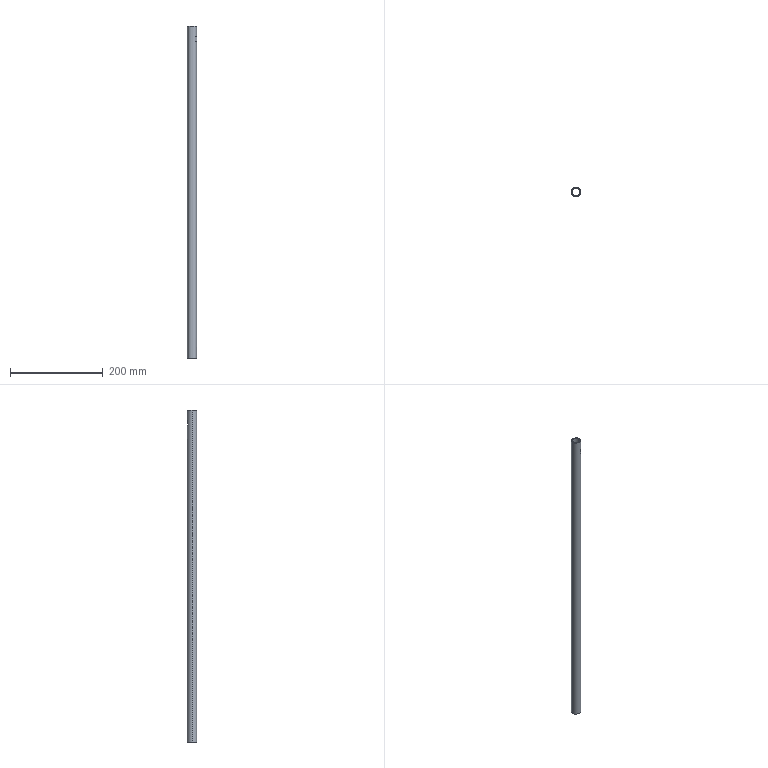Part | SolidWorks | features BaseBody 1 | 1 solid | 12 faces | box 20 x 20 x 717 mm | volume 80973 mm3 | plane 8 | cylinder 4 | commonest cylinder face diameters 16 x2 20 x2
STEP:
#1=CARTESIAN_POINT('',(-8.,0.,717.));
#2=VERTEX_POINT('',#1);
#3=CARTESIAN_POINT('',(8.,0.,717.));
#4=VERTEX_POINT('',#3);
#5=CARTESIAN_POINT('',(0.,0.,717.));
#6=DIRECTION('',(0.,0.,1.));
#7=DIRECTION('',(1.,0.,0.));
#8=AXIS2_PLACEMENT_3D('',#5,#6,#7);
#9=CIRCLE('',#8,8.);
#10=EDGE_CURVE('',#2,#4,#9,.T.);
#11=ORIENTED_EDGE('',*,*,#10,.T.);
#12=CARTESIAN_POINT('',(8.,0.,0.));
#13=VERTEX_POINT('',#12);
#14=CARTESIAN_POINT('',(8.,0.,717.));
#15=DIRECTION('',(0.,0.,-1.));
#16=VECTOR('',#15,1000.);
#17=LINE('',#14,#16);
#18=EDGE_CURVE('',#4,#13,#17,.T.);
#19=ORIENTED_EDGE('',*,*,#18,.T.);
#20=CARTESIAN_POINT('',(-8.,0.,0.));
#21=VERTEX_POINT('',#20);
#22=CARTESIAN_POINT('',(0.,0.,0.));
#23=DIRECTION('',(0.,0.,1.));
#24=DIRECTION('',(1.,0.,0.));
#25=AXIS2_PLACEMENT_3D('',#22,#23,#24);
#26=CIRCLE('',#25,8.);
#27=EDGE_CURVE('',#21,#13,#26,.T.);
#28=ORIENTED_EDGE('',*,*,#27,.F.);
#29=CARTESIAN_POINT('',(-8.,0.,717.));
#30=DIRECTION('',(0.,0.,-1.));
#31=VECTOR('',#30,1000.);
#32=LINE('',#29,#31);
#33=EDGE_CURVE('',#2,#21,#32,.T.);
#34=ORIENTED_EDGE('',*,*,#33,.F.);
#35=EDGE_LOOP('',(#11,#19,#28,#34));
#36=FACE_OUTER_BOUND('',#35,.T.);
#37=CARTESIAN_POINT('',(0.,0.,717.));
#38=DIRECTION('',(0.,0.,-1.));
#39=DIRECTION('',(-1.,0.,0.));
#40=AXIS2_PLACEMENT_3D('',#37,#38,#39);
#41=CYLINDRICAL_SURFACE('',#40,8.);
#42=ADVANCED_FACE('',(#36),#41,.F.);
#43=CARTESIAN_POINT('',(4.359,9.,684.5));
#44=VERTEX_POINT('',#43);
#45=CARTESIAN_POINT('',(-4.359,9.,684.5));
#46=VERTEX_POINT('',#45);
#47=CARTESIAN_POINT('',(0.,0.,684.5));
#48=DIRECTION('',(0.,0.,1.));
#49=DIRECTION('',(1.,0.,0.));
#50=AXIS2_PLACEMENT_3D('',#47,#48,#49);
#51=CIRCLE('',#50,10.);
#52=EDGE_CURVE('',#44,#46,#51,.T.);
#53=ORIENTED_EDGE('',*,*,#52,.F.);
#54=CARTESIAN_POINT('',(4.359,9.,694.5));
#55=VERTEX_POINT('',#54);
#56=CARTESIAN_POINT('',(4.359,9.,717.));
#57=DIRECTION('',(0.,0.,1.));
#58=VECTOR('',#57,1000.);
#59=LINE('',#56,#58);
#60=EDGE_CURVE('',#44,#55,#59,.T.);
#61=ORIENTED_EDGE('',*,*,#60,.T.);
#62=CARTESIAN_POINT('',(-4.359,9.,694.5));
#63=VERTEX_POINT('',#62);
#64=CARTESIAN_POINT('',(0.,0.,694.5));
#65=DIRECTION('',(0.,0.,1.));
#66=DIRECTION('',(1.,0.,0.));
#67=AXIS2_PLACEMENT_3D('',#64,#65,#66);
#68=CIRCLE('',#67,10.);
#69=EDGE_CURVE('',#55,#63,#68,.T.);
#70=ORIENTED_EDGE('',*,*,#69,.T.);
#71=CARTESIAN_POINT('',(-4.359,9.,717.));
#72=DIRECTION('',(0.,0.,-1.));
#73=VECTOR('',#72,1000.);
#74=LINE('',#71,#73);
#75=EDGE_CURVE('',#63,#46,#74,.T.);
#76=ORIENTED_EDGE('',*,*,#75,.T.);
#77=EDGE_LOOP('',(#53,#61,#70,#76));
#78=FACE_BOUND('',#77,.T.);
#79=CARTESIAN_POINT('',(10.,0.,717.));
#80=VERTEX_POINT('',#79);
#81=CARTESIAN_POINT('',(-10.,0.,717.));
#82=VERTEX_POINT('',#81);
#83=CARTESIAN_POINT('',(0.,0.,717.));
#84=DIRECTION('',(0.,0.,1.));
#85=DIRECTION('',(1.,0.,0.));
#86=AXIS2_PLACEMENT_3D('',#83,#84,#85);
#87=CIRCLE('',#86,10.);
#88=EDGE_CURVE('',#80,#82,#87,.T.);
#89=ORIENTED_EDGE('',*,*,#88,.F.);
#90=CARTESIAN_POINT('',(10.,0.,0.));
#91=VERTEX_POINT('',#90);
#92=CARTESIAN_POINT('',(10.,0.,717.));
#93=DIRECTION('',(0.,0.,-1.));
#94=VECTOR('',#93,1000.);
#95=LINE('',#92,#94);
#96=EDGE_CURVE('',#80,#91,#95,.T.);
#97=ORIENTED_EDGE('',*,*,#96,.T.);
#98=CARTESIAN_POINT('',(-10.,0.,0.));
#99=VERTEX_POINT('',#98);
#100=CARTESIAN_POINT('',(0.,0.,0.));
#101=DIRECTION('',(0.,0.,1.));
#102=DIRECTION('',(1.,0.,0.));
#103=AXIS2_PLACEMENT_3D('',#100,#101,#102);
#104=CIRCLE('',#103,10.);
#105=EDGE_CURVE('',#91,#99,#104,.T.);
#106=ORIENTED_EDGE('',*,*,#105,.T.);
#107=CARTESIAN_POINT('',(-10.,0.,717.));
#108=DIRECTION('',(0.,0.,-1.));
#109=VECTOR('',#108,1000.);
#110=LINE('',#107,#109);
#111=EDGE_CURVE('',#82,#99,#110,.T.);
#112=ORIENTED_EDGE('',*,*,#111,.F.);
#113=EDGE_LOOP('',(#89,#97,#106,#112));
#114=FACE_OUTER_BOUND('',#113,.T.);
#115=CARTESIAN_POINT('',(0.,0.,717.));
#116=DIRECTION('',(0.,0.,-1.));
#117=DIRECTION('',(-1.,0.,0.));
#118=AXIS2_PLACEMENT_3D('',#115,#116,#117);
#119=CYLINDRICAL_SURFACE('',#118,10.);
#120=ADVANCED_FACE('',(#78,#114),#119,.T.);
#121=CARTESIAN_POINT('',(9.974,-0.7251,694.5));
#122=VERTEX_POINT('',#121);
#123=CARTESIAN_POINT('',(5.615,-8.275,694.5));
#124=VERTEX_POINT('',#123);
#125=CARTESIAN_POINT('',(0.,0.,694.5));
#126=DIRECTION('',(0.,0.,-1.));
#127=DIRECTION('',(-1.,0.,0.));
#128=AXIS2_PLACEMENT_3D('',#125,#126,#127);
#129=CIRCLE('',#128,10.);
#130=EDGE_CURVE('',#122,#124,#129,.T.);
#131=ORIENTED_EDGE('',*,*,#130,.T.);
#132=CARTESIAN_POINT('',(12.919,4.377,694.5));
#133=DIRECTION('',(-0.5,-0.866,0.));
#134=VECTOR('',#133,1000.);
#135=LINE('',#132,#134);
#136=EDGE_CURVE('',#122,#124,#135,.T.);
#137=ORIENTED_EDGE('',*,*,#136,.F.);
#138=EDGE_LOOP('',(#131,#137));
#139=FACE_OUTER_BOUND('',#138,.T.);
#140=CARTESIAN_POINT('',(0.,0.,694.5));
#141=DIRECTION('',(0.,0.,-1.));
#142=DIRECTION('',(0.,-1.,0.));
#143=AXIS2_PLACEMENT_3D('',#140,#141,#142);
#144=PLANE('',#143);
#145=ADVANCED_FACE('',(#139),#144,.T.);
#146=CARTESIAN_POINT('',(9.974,-0.7251,684.5));
#147=VERTEX_POINT('',#146);
#148=CARTESIAN_POINT('',(5.615,-8.275,684.5));
#149=VERTEX_POINT('',#148);
#150=CARTESIAN_POINT('',(12.919,4.377,684.5));
#151=DIRECTION('',(-0.5,-0.866,0.));
#152=VECTOR('',#151,1000.);
#153=LINE('',#150,#152);
#154=EDGE_CURVE('',#147,#149,#153,.T.);
#155=ORIENTED_EDGE('',*,*,#154,.T.);
#156=CARTESIAN_POINT('',(0.,0.,684.5));
#157=DIRECTION('',(0.,0.,-1.));
#158=DIRECTION('',(-1.,0.,0.));
#159=AXIS2_PLACEMENT_3D('',#156,#157,#158);
#160=CIRCLE('',#159,10.);
#161=EDGE_CURVE('',#147,#149,#160,.T.);
#162=ORIENTED_EDGE('',*,*,#161,.F.);
#163=EDGE_LOOP('',(#155,#162));
#164=FACE_OUTER_BOUND('',#163,.T.);
#165=CARTESIAN_POINT('',(0.,0.,684.5));
#166=DIRECTION('',(0.,0.,-1.));
#167=DIRECTION('',(0.,-1.,0.));
#168=AXIS2_PLACEMENT_3D('',#165,#166,#167);
#169=PLANE('',#168);
#170=ADVANCED_FACE('',(#164),#169,.F.);
#171=ORIENTED_EDGE('',*,*,#136,.T.);
#172=CARTESIAN_POINT('',(5.615,-8.275,717.));
#173=DIRECTION('',(0.,0.,1.));
#174=VECTOR('',#173,1000.);
#175=LINE('',#172,#174);
#176=EDGE_CURVE('',#149,#124,#175,.T.);
#177=ORIENTED_EDGE('',*,*,#176,.F.);
#178=ORIENTED_EDGE('',*,*,#154,.F.);
#179=CARTESIAN_POINT('',(9.974,-0.7251,717.));
#180=DIRECTION('',(0.,0.,-1.));
#181=VECTOR('',#180,1000.);
#182=LINE('',#179,#181);
#183=EDGE_CURVE('',#122,#147,#182,.T.);
#184=ORIENTED_EDGE('',*,*,#183,.F.);
#185=EDGE_LOOP('',(#171,#177,#178,#184));
#186=FACE_OUTER_BOUND('',#185,.T.);
#187=CARTESIAN_POINT('',(12.919,4.377,684.5));
#188=DIRECTION('',(-0.866,0.5,0.));
#189=DIRECTION('',(0.,0.,1.));
#190=AXIS2_PLACEMENT_3D('',#187,#188,#189);
#191=PLANE('',#190);
#192=ADVANCED_FACE('',(#186),#191,.F.);
#193=CARTESIAN_POINT('',(-11.824,9.,694.5));
#194=DIRECTION('',(1.,0.,0.));
#195=VECTOR('',#194,1000.);
#196=LINE('',#193,#195);
#197=EDGE_CURVE('',#63,#55,#196,.T.);
#198=ORIENTED_EDGE('',*,*,#197,.F.);
#199=ORIENTED_EDGE('',*,*,#69,.F.);
#200=EDGE_LOOP('',(#198,#199));
#201=FACE_OUTER_BOUND('',#200,.T.);
#202=CARTESIAN_POINT('',(0.,0.,694.5));
#203=DIRECTION('',(0.,0.,1.));
#204=DIRECTION('',(1.,0.,0.));
#205=AXIS2_PLACEMENT_3D('',#202,#203,#204);
#206=PLANE('',#205);
#207=ADVANCED_FACE('',(#201),#206,.F.);
#208=ORIENTED_EDGE('',*,*,#52,.T.);
#209=CARTESIAN_POINT('',(-11.824,9.,684.5));
#210=DIRECTION('',(1.,0.,0.));
#211=VECTOR('',#210,1000.);
#212=LINE('',#209,#211);
#213=EDGE_CURVE('',#46,#44,#212,.T.);
#214=ORIENTED_EDGE('',*,*,#213,.T.);
#215=EDGE_LOOP('',(#208,#214));
#216=FACE_OUTER_BOUND('',#215,.T.);
#217=CARTESIAN_POINT('',(0.,0.,684.5));
#218=DIRECTION('',(0.,0.,1.));
#219=DIRECTION('',(1.,0.,0.));
#220=AXIS2_PLACEMENT_3D('',#217,#218,#219);
#221=PLANE('',#220);
#222=ADVANCED_FACE('',(#216),#221,.T.);
#223=ORIENTED_EDGE('',*,*,#197,.T.);
#224=ORIENTED_EDGE('',*,*,#60,.F.);
#225=ORIENTED_EDGE('',*,*,#213,.F.);
#226=ORIENTED_EDGE('',*,*,#75,.F.);
#227=EDGE_LOOP('',(#223,#224,#225,#226));
#228=FACE_OUTER_BOUND('',#227,.T.);
#229=CARTESIAN_POINT('',(-11.824,9.,684.5));
#230=DIRECTION('',(0.,-1.,0.));
#231=DIRECTION('',(0.,0.,-1.));
#232=AXIS2_PLACEMENT_3D('',#229,#230,#231);
#233=PLANE('',#232);
#234=ADVANCED_FACE('',(#228),#233,.F.);
#235=ORIENTED_EDGE('',*,*,#27,.T.);
#236=CARTESIAN_POINT('',(0.,0.,0.));
#237=DIRECTION('',(0.,0.,1.));
#238=DIRECTION('',(1.,0.,0.));
#239=AXIS2_PLACEMENT_3D('',#236,#237,#238);
#240=CIRCLE('',#239,8.);
#241=EDGE_CURVE('',#13,#21,#240,.T.);
#242=ORIENTED_EDGE('',*,*,#241,.T.);
#243=EDGE_LOOP('',(#235,#242));
#244=FACE_BOUND('',#243,.T.);
#245=CARTESIAN_POINT('',(0.,0.,0.));
#246=DIRECTION('',(0.,0.,1.));
#247=DIRECTION('',(1.,0.,0.));
#248=AXIS2_PLACEMENT_3D('',#245,#246,#247);
#249=CIRCLE('',#248,10.);
#250=EDGE_CURVE('',#99,#91,#249,.T.);
#251=ORIENTED_EDGE('',*,*,#250,.F.);
#252=ORIENTED_EDGE('',*,*,#105,.F.);
#253=EDGE_LOOP('',(#251,#252));
#254=FACE_OUTER_BOUND('',#253,.T.);
#255=CARTESIAN_POINT('',(0.,0.,0.));
#256=DIRECTION('',(0.,0.,1.));
#257=DIRECTION('',(1.,0.,0.));
#258=AXIS2_PLACEMENT_3D('',#255,#256,#257);
#259=PLANE('',#258);
#260=ADVANCED_FACE('',(#244,#254),#259,.F.);
#261=ORIENTED_EDGE('',*,*,#10,.F.);
#262=CARTESIAN_POINT('',(0.,0.,717.));
#263=DIRECTION('',(0.,0.,1.));
#264=DIRECTION('',(1.,0.,0.));
#265=AXIS2_PLACEMENT_3D('',#262,#263,#264);
#266=CIRCLE('',#265,8.);
#267=EDGE_CURVE('',#4,#2,#266,.T.);
#268=ORIENTED_EDGE('',*,*,#267,.F.);
#269=EDGE_LOOP('',(#261,#268));
#270=FACE_BOUND('',#269,.T.);
#271=CARTESIAN_POINT('',(0.,0.,717.));
#272=DIRECTION('',(0.,0.,1.));
#273=DIRECTION('',(1.,0.,0.));
#274=AXIS2_PLACEMENT_3D('',#271,#272,#273);
#275=CIRCLE('',#274,10.);
#276=EDGE_CURVE('',#82,#80,#275,.T.);
#277=ORIENTED_EDGE('',*,*,#276,.T.);
#278=ORIENTED_EDGE('',*,*,#88,.T.);
#279=EDGE_LOOP('',(#277,#278));
#280=FACE_OUTER_BOUND('',#279,.T.);
#281=CARTESIAN_POINT('',(0.,0.,717.));
#282=DIRECTION('',(0.,0.,1.));
#283=DIRECTION('',(1.,0.,0.));
#284=AXIS2_PLACEMENT_3D('',#281,#282,#283);
#285=PLANE('',#284);
#286=ADVANCED_FACE('',(#270,#280),#285,.T.);
#287=ORIENTED_EDGE('',*,*,#96,.F.);
#288=ORIENTED_EDGE('',*,*,#276,.F.);
#289=ORIENTED_EDGE('',*,*,#111,.T.);
#290=ORIENTED_EDGE('',*,*,#250,.T.);
#291=EDGE_LOOP('',(#287,#288,#289,#290));
#292=FACE_OUTER_BOUND('',#291,.T.);
#293=ORIENTED_EDGE('',*,*,#183,.T.);
#294=ORIENTED_EDGE('',*,*,#161,.T.);
#295=ORIENTED_EDGE('',*,*,#176,.T.);
#296=ORIENTED_EDGE('',*,*,#130,.F.);
#297=EDGE_LOOP('',(#293,#294,#295,#296));
#298=FACE_BOUND('',#297,.T.);
#299=CARTESIAN_POINT('',(0.,0.,717.));
#300=DIRECTION('',(0.,0.,-1.));
#301=DIRECTION('',(-1.,0.,0.));
#302=AXIS2_PLACEMENT_3D('',#299,#300,#301);
#303=CYLINDRICAL_SURFACE('',#302,10.);
#304=ADVANCED_FACE('',(#292,#298),#303,.T.);
#305=ORIENTED_EDGE('',*,*,#18,.F.);
#306=ORIENTED_EDGE('',*,*,#267,.T.);
#307=ORIENTED_EDGE('',*,*,#33,.T.);
#308=ORIENTED_EDGE('',*,*,#241,.F.);
#309=EDGE_LOOP('',(#305,#306,#307,#308));
#310=FACE_OUTER_BOUND('',#309,.T.);
#311=CARTESIAN_POINT('',(0.,0.,717.));
#312=DIRECTION('',(0.,0.,-1.));
#313=DIRECTION('',(-1.,0.,0.));
#314=AXIS2_PLACEMENT_3D('',#311,#312,#313);
#315=CYLINDRICAL_SURFACE('',#314,8.);
#316=ADVANCED_FACE('',(#310),#315,.F.);
#317=CLOSED_SHELL('',(#42,#120,#145,#170,#192,#207,#222,#234,#260,#286,#304,#316));
#318=MANIFOLD_SOLID_BREP('',#317);
#319=CARTESIAN_POINT('',(0.,0.,0.));
#320=DIRECTION('',(0.,0.,1.));
#321=DIRECTION('',(1.,0.,0.));
#322=AXIS2_PLACEMENT_3D('',#319,#320,#321);
#323=(LENGTH_UNIT()NAMED_UNIT(*)SI_UNIT(.MILLI.,.METRE.));
#324=UNCERTAINTY_MEASURE_WITH_UNIT(LENGTH_MEASURE(0.00001),#323,'','');
#325=(NAMED_UNIT(*)PLANE_ANGLE_UNIT()SI_UNIT($,.RADIAN.));
#326=(NAMED_UNIT(*)SI_UNIT($,.STERADIAN.)SOLID_ANGLE_UNIT());
#327=(GEOMETRIC_REPRESENTATION_CONTEXT(3)GLOBAL_UNCERTAINTY_ASSIGNED_CONTEXT((#324))GLOBAL_UNIT_ASSIGNED_CONTEXT((#323,#325,#326))REPRESENTATION_CONTEXT('',''));
#328=ADVANCED_BREP_SHAPE_REPRESENTATION('',(#318,#322),#327);